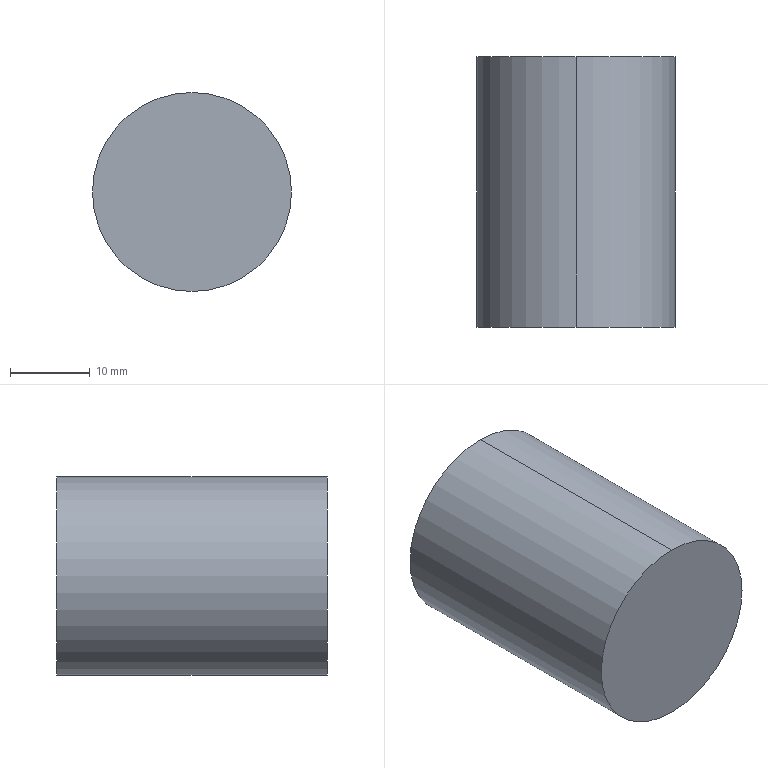Part | SolidWorks | features Extrusion 1 | 1 solid | 4 faces | box 25 x 34 x 25 mm | volume 16690 mm3 | cylinder 2 | plane 2 | commonest cylinder face diameters 25 x2
STEP:
#1=CARTESIAN_POINT('',(0.,34.,12.5));
#2=VERTEX_POINT('',#1);
#3=CARTESIAN_POINT('',(0.,34.,-12.5));
#4=VERTEX_POINT('',#3);
#5=CARTESIAN_POINT('',(0.,34.,0.));
#6=DIRECTION('',(0.,1.,0.));
#7=DIRECTION('',(0.,0.,1.));
#8=AXIS2_PLACEMENT_3D('',#5,#6,#7);
#9=CIRCLE('',#8,12.5);
#10=EDGE_CURVE('',#2,#4,#9,.T.);
#11=ORIENTED_EDGE('',*,*,#10,.F.);
#12=CARTESIAN_POINT('',(0.,0.,12.5));
#13=VERTEX_POINT('',#12);
#14=CARTESIAN_POINT('',(0.,34.,12.5));
#15=DIRECTION('',(0.,-1.,0.));
#16=VECTOR('',#15,1000.);
#17=LINE('',#14,#16);
#18=EDGE_CURVE('',#2,#13,#17,.T.);
#19=ORIENTED_EDGE('',*,*,#18,.T.);
#20=CARTESIAN_POINT('',(0.,0.,-12.5));
#21=VERTEX_POINT('',#20);
#22=CARTESIAN_POINT('',(0.,0.,0.));
#23=DIRECTION('',(0.,1.,0.));
#24=DIRECTION('',(0.,0.,1.));
#25=AXIS2_PLACEMENT_3D('',#22,#23,#24);
#26=CIRCLE('',#25,12.5);
#27=EDGE_CURVE('',#13,#21,#26,.T.);
#28=ORIENTED_EDGE('',*,*,#27,.T.);
#29=CARTESIAN_POINT('',(0.,34.,-12.5));
#30=DIRECTION('',(0.,-1.,0.));
#31=VECTOR('',#30,1000.);
#32=LINE('',#29,#31);
#33=EDGE_CURVE('',#4,#21,#32,.T.);
#34=ORIENTED_EDGE('',*,*,#33,.F.);
#35=EDGE_LOOP('',(#11,#19,#28,#34));
#36=FACE_OUTER_BOUND('',#35,.T.);
#37=CARTESIAN_POINT('',(0.,34.,0.));
#38=DIRECTION('',(0.,-1.,0.));
#39=DIRECTION('',(0.,0.,-1.));
#40=AXIS2_PLACEMENT_3D('',#37,#38,#39);
#41=CYLINDRICAL_SURFACE('',#40,12.5);
#42=ADVANCED_FACE('',(#36),#41,.T.);
#43=ORIENTED_EDGE('',*,*,#18,.F.);
#44=CARTESIAN_POINT('',(0.,34.,0.));
#45=DIRECTION('',(0.,1.,0.));
#46=DIRECTION('',(0.,0.,1.));
#47=AXIS2_PLACEMENT_3D('',#44,#45,#46);
#48=CIRCLE('',#47,12.5);
#49=EDGE_CURVE('',#4,#2,#48,.T.);
#50=ORIENTED_EDGE('',*,*,#49,.F.);
#51=ORIENTED_EDGE('',*,*,#33,.T.);
#52=CARTESIAN_POINT('',(0.,0.,0.));
#53=DIRECTION('',(0.,1.,0.));
#54=DIRECTION('',(0.,0.,1.));
#55=AXIS2_PLACEMENT_3D('',#52,#53,#54);
#56=CIRCLE('',#55,12.5);
#57=EDGE_CURVE('',#21,#13,#56,.T.);
#58=ORIENTED_EDGE('',*,*,#57,.T.);
#59=EDGE_LOOP('',(#43,#50,#51,#58));
#60=FACE_OUTER_BOUND('',#59,.T.);
#61=CARTESIAN_POINT('',(0.,34.,0.));
#62=DIRECTION('',(0.,-1.,0.));
#63=DIRECTION('',(0.,0.,-1.));
#64=AXIS2_PLACEMENT_3D('',#61,#62,#63);
#65=CYLINDRICAL_SURFACE('',#64,12.5);
#66=ADVANCED_FACE('',(#60),#65,.T.);
#67=ORIENTED_EDGE('',*,*,#49,.T.);
#68=ORIENTED_EDGE('',*,*,#10,.T.);
#69=EDGE_LOOP('',(#67,#68));
#70=FACE_OUTER_BOUND('',#69,.T.);
#71=CARTESIAN_POINT('',(0.,34.,0.));
#72=DIRECTION('',(0.,1.,0.));
#73=DIRECTION('',(0.,0.,1.));
#74=AXIS2_PLACEMENT_3D('',#71,#72,#73);
#75=PLANE('',#74);
#76=ADVANCED_FACE('',(#70),#75,.T.);
#77=ORIENTED_EDGE('',*,*,#57,.F.);
#78=ORIENTED_EDGE('',*,*,#27,.F.);
#79=EDGE_LOOP('',(#77,#78));
#80=FACE_OUTER_BOUND('',#79,.T.);
#81=CARTESIAN_POINT('',(0.,0.,0.));
#82=DIRECTION('',(0.,1.,0.));
#83=DIRECTION('',(0.,0.,1.));
#84=AXIS2_PLACEMENT_3D('',#81,#82,#83);
#85=PLANE('',#84);
#86=ADVANCED_FACE('',(#80),#85,.F.);
#87=CLOSED_SHELL('',(#42,#66,#76,#86));
#88=MANIFOLD_SOLID_BREP('',#87);
#89=CARTESIAN_POINT('',(0.,0.,0.));
#90=DIRECTION('',(0.,0.,1.));
#91=DIRECTION('',(1.,0.,0.));
#92=AXIS2_PLACEMENT_3D('',#89,#90,#91);
#93=(LENGTH_UNIT()NAMED_UNIT(*)SI_UNIT(.MILLI.,.METRE.));
#94=UNCERTAINTY_MEASURE_WITH_UNIT(LENGTH_MEASURE(0.00001),#93,'','');
#95=(NAMED_UNIT(*)PLANE_ANGLE_UNIT()SI_UNIT($,.RADIAN.));
#96=(NAMED_UNIT(*)SI_UNIT($,.STERADIAN.)SOLID_ANGLE_UNIT());
#97=(GEOMETRIC_REPRESENTATION_CONTEXT(3)GLOBAL_UNCERTAINTY_ASSIGNED_CONTEXT((#94))GLOBAL_UNIT_ASSIGNED_CONTEXT((#93,#95,#96))REPRESENTATION_CONTEXT('',''));
#98=ADVANCED_BREP_SHAPE_REPRESENTATION('',(#88,#92),#97);